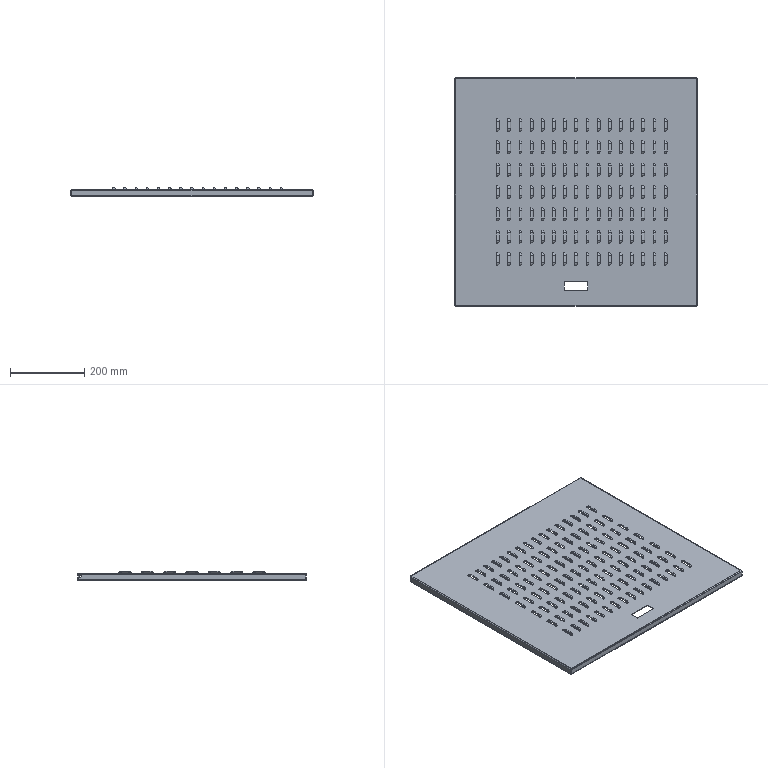Part | STEP file | Side door panel upper V1.201001 | 1 solid | 1646 faces | box 651 x 615 x 25 mm | volume 711845 mm3 | cylinder 468 | torus 448 | sphere 448 | plane 266 | spline 16 | commonest cylinder face diameters 1 x112 4 x112 12 x112 15 x112 3 x8 6 x8